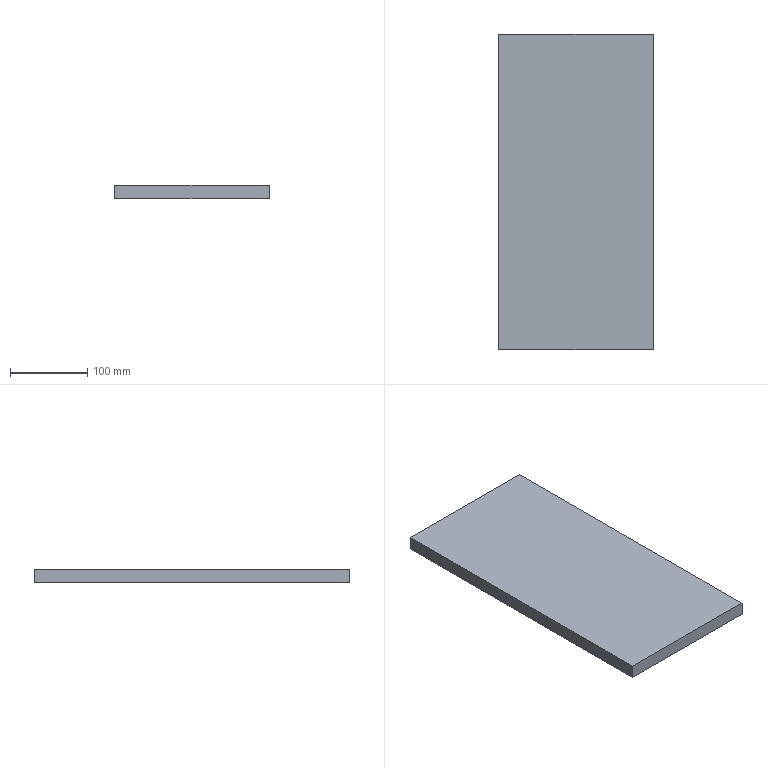Part | STEP file | Superstructure_3 | 1 solid | 6 faces | box 200 x 408 x 18 mm | volume 1468800 mm3 | plane 6
STEP:
#1=CARTESIAN_POINT('',(0.,0.,0.));
#2=DIRECTION('',(0.,0.,1.));
#3=DIRECTION('',(1.,0.,0.));
#4=AXIS2_PLACEMENT_3D('',#1,#2,#3);
#5=CARTESIAN_POINT('',(-100.,204.,9.));
#6=VERTEX_POINT('',#5);
#7=CARTESIAN_POINT('',(-100.,-204.,9.));
#8=VERTEX_POINT('',#7);
#9=CARTESIAN_POINT('',(-100.,204.,9.));
#10=DIRECTION('',(0.,-1.,0.));
#11=VECTOR('',#10,1.);
#12=LINE('',#9,#11);
#13=CARTESIAN_POINT('',(-100.,204.,9.));
#14=DIRECTION('',(1.,0.,0.));
#15=DIRECTION('',(0.,0.,-1.));
#16=AXIS2_PLACEMENT_3D('',#13,#14,#15);
#17=PLANE('',#16);
#18=CARTESIAN_POINT('',(0.,0.));
#19=DIRECTION('',(0.,-1.));
#20=VECTOR('',#19,1.);
#21=LINE('',#18,#20);
#22=(GEOMETRIC_REPRESENTATION_CONTEXT(2)PARAMETRIC_REPRESENTATION_CONTEXT()REPRESENTATION_CONTEXT('',''));
#23=DEFINITIONAL_REPRESENTATION('',(#21),#22);
#24=PCURVE('',#17,#23);
#25=CARTESIAN_POINT('',(100.,204.,9.));
#26=DIRECTION('',(0.,0.,-1.));
#27=DIRECTION('',(-1.,0.,0.));
#28=AXIS2_PLACEMENT_3D('',#25,#26,#27);
#29=PLANE('',#28);
#30=CARTESIAN_POINT('',(200.,0.));
#31=DIRECTION('',(0.,-1.));
#32=VECTOR('',#31,1.);
#33=LINE('',#30,#32);
#34=(GEOMETRIC_REPRESENTATION_CONTEXT(2)PARAMETRIC_REPRESENTATION_CONTEXT()REPRESENTATION_CONTEXT('',''));
#35=DEFINITIONAL_REPRESENTATION('',(#33),#34);
#36=PCURVE('',#29,#35);
#37=SURFACE_CURVE('',#12,(#24,#36),.PCURVE_S1.);
#38=EDGE_CURVE('',#6,#8,#37,.T.);
#39=ORIENTED_EDGE('',*,*,#38,.T.);
#40=CARTESIAN_POINT('',(-100.,-204.,-9.));
#41=VERTEX_POINT('',#40);
#42=CARTESIAN_POINT('',(-100.,-204.,9.));
#43=DIRECTION('',(0.,0.,-1.));
#44=VECTOR('',#43,1.);
#45=LINE('',#42,#44);
#46=CARTESIAN_POINT('',(0.,-408.));
#47=DIRECTION('',(1.,0.));
#48=VECTOR('',#47,1.);
#49=LINE('',#46,#48);
#50=(GEOMETRIC_REPRESENTATION_CONTEXT(2)PARAMETRIC_REPRESENTATION_CONTEXT()REPRESENTATION_CONTEXT('',''));
#51=DEFINITIONAL_REPRESENTATION('',(#49),#50);
#52=PCURVE('',#17,#51);
#53=CARTESIAN_POINT('',(0.,-204.,0.));
#54=DIRECTION('',(0.,1.,0.));
#55=DIRECTION('',(0.,0.,1.));
#56=AXIS2_PLACEMENT_3D('',#53,#54,#55);
#57=PLANE('',#56);
#58=CARTESIAN_POINT('',(9.,-100.));
#59=DIRECTION('',(-1.,0.));
#60=VECTOR('',#59,1.);
#61=LINE('',#58,#60);
#62=(GEOMETRIC_REPRESENTATION_CONTEXT(2)PARAMETRIC_REPRESENTATION_CONTEXT()REPRESENTATION_CONTEXT('',''));
#63=DEFINITIONAL_REPRESENTATION('',(#61),#62);
#64=PCURVE('',#57,#63);
#65=SURFACE_CURVE('',#45,(#52,#64),.PCURVE_S1.);
#66=EDGE_CURVE('',#8,#41,#65,.T.);
#67=ORIENTED_EDGE('',*,*,#66,.T.);
#68=CARTESIAN_POINT('',(-100.,204.,-9.));
#69=VERTEX_POINT('',#68);
#70=CARTESIAN_POINT('',(-100.,204.,-9.));
#71=DIRECTION('',(0.,-1.,0.));
#72=VECTOR('',#71,1.);
#73=LINE('',#70,#72);
#74=CARTESIAN_POINT('',(18.,0.));
#75=DIRECTION('',(0.,-1.));
#76=VECTOR('',#75,1.);
#77=LINE('',#74,#76);
#78=(GEOMETRIC_REPRESENTATION_CONTEXT(2)PARAMETRIC_REPRESENTATION_CONTEXT()REPRESENTATION_CONTEXT('',''));
#79=DEFINITIONAL_REPRESENTATION('',(#77),#78);
#80=PCURVE('',#17,#79);
#81=CARTESIAN_POINT('',(-100.,204.,-9.));
#82=DIRECTION('',(0.,0.,1.));
#83=DIRECTION('',(1.,0.,0.));
#84=AXIS2_PLACEMENT_3D('',#81,#82,#83);
#85=PLANE('',#84);
#86=CARTESIAN_POINT('',(0.,0.));
#87=DIRECTION('',(0.,-1.));
#88=VECTOR('',#87,1.);
#89=LINE('',#86,#88);
#90=(GEOMETRIC_REPRESENTATION_CONTEXT(2)PARAMETRIC_REPRESENTATION_CONTEXT()REPRESENTATION_CONTEXT('',''));
#91=DEFINITIONAL_REPRESENTATION('',(#89),#90);
#92=PCURVE('',#85,#91);
#93=SURFACE_CURVE('',#73,(#80,#92),.PCURVE_S1.);
#94=EDGE_CURVE('',#69,#41,#93,.T.);
#95=ORIENTED_EDGE('',*,*,#94,.F.);
#96=CARTESIAN_POINT('',(-100.,204.,9.));
#97=DIRECTION('',(0.,0.,-1.));
#98=VECTOR('',#97,1.);
#99=LINE('',#96,#98);
#100=CARTESIAN_POINT('',(0.,0.));
#101=DIRECTION('',(1.,0.));
#102=VECTOR('',#101,1.);
#103=LINE('',#100,#102);
#104=(GEOMETRIC_REPRESENTATION_CONTEXT(2)PARAMETRIC_REPRESENTATION_CONTEXT()REPRESENTATION_CONTEXT('',''));
#105=DEFINITIONAL_REPRESENTATION('',(#103),#104);
#106=PCURVE('',#17,#105);
#107=CARTESIAN_POINT('',(0.,204.,0.));
#108=DIRECTION('',(0.,1.,0.));
#109=DIRECTION('',(0.,0.,1.));
#110=AXIS2_PLACEMENT_3D('',#107,#108,#109);
#111=PLANE('',#110);
#112=CARTESIAN_POINT('',(9.,-100.));
#113=DIRECTION('',(-1.,0.));
#114=VECTOR('',#113,1.);
#115=LINE('',#112,#114);
#116=(GEOMETRIC_REPRESENTATION_CONTEXT(2)PARAMETRIC_REPRESENTATION_CONTEXT()REPRESENTATION_CONTEXT('',''));
#117=DEFINITIONAL_REPRESENTATION('',(#115),#116);
#118=PCURVE('',#111,#117);
#119=SURFACE_CURVE('',#99,(#106,#118),.PCURVE_S1.);
#120=EDGE_CURVE('',#6,#69,#119,.T.);
#121=ORIENTED_EDGE('',*,*,#120,.F.);
#122=EDGE_LOOP('',(#39,#67,#95,#121));
#123=FACE_BOUND('',#122,.F.);
#124=ADVANCED_FACE('',(#123),#17,.F.);
#125=ORIENTED_EDGE('',*,*,#94,.T.);
#126=CARTESIAN_POINT('',(100.,-204.,-9.));
#127=VERTEX_POINT('',#126);
#128=CARTESIAN_POINT('',(-100.,-204.,-9.));
#129=DIRECTION('',(1.,0.,0.));
#130=VECTOR('',#129,1.);
#131=LINE('',#128,#130);
#132=CARTESIAN_POINT('',(0.,-408.));
#133=DIRECTION('',(1.,0.));
#134=VECTOR('',#133,1.);
#135=LINE('',#132,#134);
#136=(GEOMETRIC_REPRESENTATION_CONTEXT(2)PARAMETRIC_REPRESENTATION_CONTEXT()REPRESENTATION_CONTEXT('',''));
#137=DEFINITIONAL_REPRESENTATION('',(#135),#136);
#138=PCURVE('',#85,#137);
#139=CARTESIAN_POINT('',(-9.,-100.));
#140=DIRECTION('',(0.,1.));
#141=VECTOR('',#140,1.);
#142=LINE('',#139,#141);
#143=(GEOMETRIC_REPRESENTATION_CONTEXT(2)PARAMETRIC_REPRESENTATION_CONTEXT()REPRESENTATION_CONTEXT('',''));
#144=DEFINITIONAL_REPRESENTATION('',(#142),#143);
#145=PCURVE('',#57,#144);
#146=SURFACE_CURVE('',#131,(#138,#145),.PCURVE_S1.);
#147=EDGE_CURVE('',#41,#127,#146,.T.);
#148=ORIENTED_EDGE('',*,*,#147,.T.);
#149=CARTESIAN_POINT('',(100.,204.,-9.));
#150=VERTEX_POINT('',#149);
#151=CARTESIAN_POINT('',(100.,204.,-9.));
#152=DIRECTION('',(0.,-1.,0.));
#153=VECTOR('',#152,1.);
#154=LINE('',#151,#153);
#155=CARTESIAN_POINT('',(200.,0.));
#156=DIRECTION('',(0.,-1.));
#157=VECTOR('',#156,1.);
#158=LINE('',#155,#157);
#159=(GEOMETRIC_REPRESENTATION_CONTEXT(2)PARAMETRIC_REPRESENTATION_CONTEXT()REPRESENTATION_CONTEXT('',''));
#160=DEFINITIONAL_REPRESENTATION('',(#158),#159);
#161=PCURVE('',#85,#160);
#162=CARTESIAN_POINT('',(100.,204.,-9.));
#163=DIRECTION('',(-1.,0.,0.));
#164=DIRECTION('',(0.,0.,1.));
#165=AXIS2_PLACEMENT_3D('',#162,#163,#164);
#166=PLANE('',#165);
#167=CARTESIAN_POINT('',(0.,0.));
#168=DIRECTION('',(0.,-1.));
#169=VECTOR('',#168,1.);
#170=LINE('',#167,#169);
#171=(GEOMETRIC_REPRESENTATION_CONTEXT(2)PARAMETRIC_REPRESENTATION_CONTEXT()REPRESENTATION_CONTEXT('',''));
#172=DEFINITIONAL_REPRESENTATION('',(#170),#171);
#173=PCURVE('',#166,#172);
#174=SURFACE_CURVE('',#154,(#161,#173),.PCURVE_S1.);
#175=EDGE_CURVE('',#150,#127,#174,.T.);
#176=ORIENTED_EDGE('',*,*,#175,.F.);
#177=CARTESIAN_POINT('',(-100.,204.,-9.));
#178=DIRECTION('',(1.,0.,0.));
#179=VECTOR('',#178,1.);
#180=LINE('',#177,#179);
#181=CARTESIAN_POINT('',(0.,0.));
#182=DIRECTION('',(1.,0.));
#183=VECTOR('',#182,1.);
#184=LINE('',#181,#183);
#185=(GEOMETRIC_REPRESENTATION_CONTEXT(2)PARAMETRIC_REPRESENTATION_CONTEXT()REPRESENTATION_CONTEXT('',''));
#186=DEFINITIONAL_REPRESENTATION('',(#184),#185);
#187=PCURVE('',#85,#186);
#188=CARTESIAN_POINT('',(-9.,-100.));
#189=DIRECTION('',(0.,1.));
#190=VECTOR('',#189,1.);
#191=LINE('',#188,#190);
#192=(GEOMETRIC_REPRESENTATION_CONTEXT(2)PARAMETRIC_REPRESENTATION_CONTEXT()REPRESENTATION_CONTEXT('',''));
#193=DEFINITIONAL_REPRESENTATION('',(#191),#192);
#194=PCURVE('',#111,#193);
#195=SURFACE_CURVE('',#180,(#187,#194),.PCURVE_S1.);
#196=EDGE_CURVE('',#69,#150,#195,.T.);
#197=ORIENTED_EDGE('',*,*,#196,.F.);
#198=EDGE_LOOP('',(#125,#148,#176,#197));
#199=FACE_BOUND('',#198,.F.);
#200=ADVANCED_FACE('',(#199),#85,.F.);
#201=ORIENTED_EDGE('',*,*,#175,.T.);
#202=CARTESIAN_POINT('',(100.,-204.,9.));
#203=VERTEX_POINT('',#202);
#204=CARTESIAN_POINT('',(100.,-204.,-9.));
#205=DIRECTION('',(0.,0.,1.));
#206=VECTOR('',#205,1.);
#207=LINE('',#204,#206);
#208=CARTESIAN_POINT('',(0.,-408.));
#209=DIRECTION('',(1.,0.));
#210=VECTOR('',#209,1.);
#211=LINE('',#208,#210);
#212=(GEOMETRIC_REPRESENTATION_CONTEXT(2)PARAMETRIC_REPRESENTATION_CONTEXT()REPRESENTATION_CONTEXT('',''));
#213=DEFINITIONAL_REPRESENTATION('',(#211),#212);
#214=PCURVE('',#166,#213);
#215=CARTESIAN_POINT('',(-9.,100.));
#216=DIRECTION('',(1.,0.));
#217=VECTOR('',#216,1.);
#218=LINE('',#215,#217);
#219=(GEOMETRIC_REPRESENTATION_CONTEXT(2)PARAMETRIC_REPRESENTATION_CONTEXT()REPRESENTATION_CONTEXT('',''));
#220=DEFINITIONAL_REPRESENTATION('',(#218),#219);
#221=PCURVE('',#57,#220);
#222=SURFACE_CURVE('',#207,(#214,#221),.PCURVE_S1.);
#223=EDGE_CURVE('',#127,#203,#222,.T.);
#224=ORIENTED_EDGE('',*,*,#223,.T.);
#225=CARTESIAN_POINT('',(100.,204.,9.));
#226=VERTEX_POINT('',#225);
#227=CARTESIAN_POINT('',(100.,204.,9.));
#228=DIRECTION('',(0.,-1.,0.));
#229=VECTOR('',#228,1.);
#230=LINE('',#227,#229);
#231=CARTESIAN_POINT('',(18.,0.));
#232=DIRECTION('',(0.,-1.));
#233=VECTOR('',#232,1.);
#234=LINE('',#231,#233);
#235=(GEOMETRIC_REPRESENTATION_CONTEXT(2)PARAMETRIC_REPRESENTATION_CONTEXT()REPRESENTATION_CONTEXT('',''));
#236=DEFINITIONAL_REPRESENTATION('',(#234),#235);
#237=PCURVE('',#166,#236);
#238=CARTESIAN_POINT('',(0.,0.));
#239=DIRECTION('',(0.,-1.));
#240=VECTOR('',#239,1.);
#241=LINE('',#238,#240);
#242=(GEOMETRIC_REPRESENTATION_CONTEXT(2)PARAMETRIC_REPRESENTATION_CONTEXT()REPRESENTATION_CONTEXT('',''));
#243=DEFINITIONAL_REPRESENTATION('',(#241),#242);
#244=PCURVE('',#29,#243);
#245=SURFACE_CURVE('',#230,(#237,#244),.PCURVE_S1.);
#246=EDGE_CURVE('',#226,#203,#245,.T.);
#247=ORIENTED_EDGE('',*,*,#246,.F.);
#248=CARTESIAN_POINT('',(100.,204.,-9.));
#249=DIRECTION('',(0.,0.,1.));
#250=VECTOR('',#249,1.);
#251=LINE('',#248,#250);
#252=CARTESIAN_POINT('',(0.,0.));
#253=DIRECTION('',(1.,0.));
#254=VECTOR('',#253,1.);
#255=LINE('',#252,#254);
#256=(GEOMETRIC_REPRESENTATION_CONTEXT(2)PARAMETRIC_REPRESENTATION_CONTEXT()REPRESENTATION_CONTEXT('',''));
#257=DEFINITIONAL_REPRESENTATION('',(#255),#256);
#258=PCURVE('',#166,#257);
#259=CARTESIAN_POINT('',(-9.,100.));
#260=DIRECTION('',(1.,0.));
#261=VECTOR('',#260,1.);
#262=LINE('',#259,#261);
#263=(GEOMETRIC_REPRESENTATION_CONTEXT(2)PARAMETRIC_REPRESENTATION_CONTEXT()REPRESENTATION_CONTEXT('',''));
#264=DEFINITIONAL_REPRESENTATION('',(#262),#263);
#265=PCURVE('',#111,#264);
#266=SURFACE_CURVE('',#251,(#258,#265),.PCURVE_S1.);
#267=EDGE_CURVE('',#150,#226,#266,.T.);
#268=ORIENTED_EDGE('',*,*,#267,.F.);
#269=EDGE_LOOP('',(#201,#224,#247,#268));
#270=FACE_BOUND('',#269,.F.);
#271=ADVANCED_FACE('',(#270),#166,.F.);
#272=ORIENTED_EDGE('',*,*,#246,.T.);
#273=CARTESIAN_POINT('',(100.,-204.,9.));
#274=DIRECTION('',(-1.,0.,0.));
#275=VECTOR('',#274,1.);
#276=LINE('',#273,#275);
#277=CARTESIAN_POINT('',(0.,-408.));
#278=DIRECTION('',(1.,0.));
#279=VECTOR('',#278,1.);
#280=LINE('',#277,#279);
#281=(GEOMETRIC_REPRESENTATION_CONTEXT(2)PARAMETRIC_REPRESENTATION_CONTEXT()REPRESENTATION_CONTEXT('',''));
#282=DEFINITIONAL_REPRESENTATION('',(#280),#281);
#283=PCURVE('',#29,#282);
#284=CARTESIAN_POINT('',(9.,100.));
#285=DIRECTION('',(0.,-1.));
#286=VECTOR('',#285,1.);
#287=LINE('',#284,#286);
#288=(GEOMETRIC_REPRESENTATION_CONTEXT(2)PARAMETRIC_REPRESENTATION_CONTEXT()REPRESENTATION_CONTEXT('',''));
#289=DEFINITIONAL_REPRESENTATION('',(#287),#288);
#290=PCURVE('',#57,#289);
#291=SURFACE_CURVE('',#276,(#283,#290),.PCURVE_S1.);
#292=EDGE_CURVE('',#203,#8,#291,.T.);
#293=ORIENTED_EDGE('',*,*,#292,.T.);
#294=ORIENTED_EDGE('',*,*,#38,.F.);
#295=CARTESIAN_POINT('',(100.,204.,9.));
#296=DIRECTION('',(-1.,0.,0.));
#297=VECTOR('',#296,1.);
#298=LINE('',#295,#297);
#299=CARTESIAN_POINT('',(0.,0.));
#300=DIRECTION('',(1.,0.));
#301=VECTOR('',#300,1.);
#302=LINE('',#299,#301);
#303=(GEOMETRIC_REPRESENTATION_CONTEXT(2)PARAMETRIC_REPRESENTATION_CONTEXT()REPRESENTATION_CONTEXT('',''));
#304=DEFINITIONAL_REPRESENTATION('',(#302),#303);
#305=PCURVE('',#29,#304);
#306=CARTESIAN_POINT('',(9.,100.));
#307=DIRECTION('',(0.,-1.));
#308=VECTOR('',#307,1.);
#309=LINE('',#306,#308);
#310=(GEOMETRIC_REPRESENTATION_CONTEXT(2)PARAMETRIC_REPRESENTATION_CONTEXT()REPRESENTATION_CONTEXT('',''));
#311=DEFINITIONAL_REPRESENTATION('',(#309),#310);
#312=PCURVE('',#111,#311);
#313=SURFACE_CURVE('',#298,(#305,#312),.PCURVE_S1.);
#314=EDGE_CURVE('',#226,#6,#313,.T.);
#315=ORIENTED_EDGE('',*,*,#314,.F.);
#316=EDGE_LOOP('',(#272,#293,#294,#315));
#317=FACE_BOUND('',#316,.F.);
#318=ADVANCED_FACE('',(#317),#29,.F.);
#319=ORIENTED_EDGE('',*,*,#120,.T.);
#320=ORIENTED_EDGE('',*,*,#196,.T.);
#321=ORIENTED_EDGE('',*,*,#267,.T.);
#322=ORIENTED_EDGE('',*,*,#314,.T.);
#323=EDGE_LOOP('',(#319,#320,#321,#322));
#324=FACE_BOUND('',#323,.F.);
#325=ADVANCED_FACE('',(#324),#111,.T.);
#326=ORIENTED_EDGE('',*,*,#66,.T.);
#327=ORIENTED_EDGE('',*,*,#147,.T.);
#328=ORIENTED_EDGE('',*,*,#223,.T.);
#329=ORIENTED_EDGE('',*,*,#292,.T.);
#330=EDGE_LOOP('',(#326,#327,#328,#329));
#331=FACE_BOUND('',#330,.T.);
#332=ADVANCED_FACE('',(#331),#57,.F.);
#333=CLOSED_SHELL('',(#124,#200,#271,#318,#325,#332));
#334=MANIFOLD_SOLID_BREP('',#333);
#335=(LENGTH_UNIT()NAMED_UNIT(*)SI_UNIT(.MILLI.,.METRE.));
#336=UNCERTAINTY_MEASURE_WITH_UNIT(LENGTH_MEASURE(0.0000001),#335,'','');
#337=(NAMED_UNIT(*)PLANE_ANGLE_UNIT()SI_UNIT($,.RADIAN.));
#338=(NAMED_UNIT(*)SI_UNIT($,.STERADIAN.)SOLID_ANGLE_UNIT());
#339=(GEOMETRIC_REPRESENTATION_CONTEXT(3)GLOBAL_UNCERTAINTY_ASSIGNED_CONTEXT((#336))GLOBAL_UNIT_ASSIGNED_CONTEXT((#335,#337,#338))REPRESENTATION_CONTEXT('',''));
#340=ADVANCED_BREP_SHAPE_REPRESENTATION('',(#4,#334),#339);